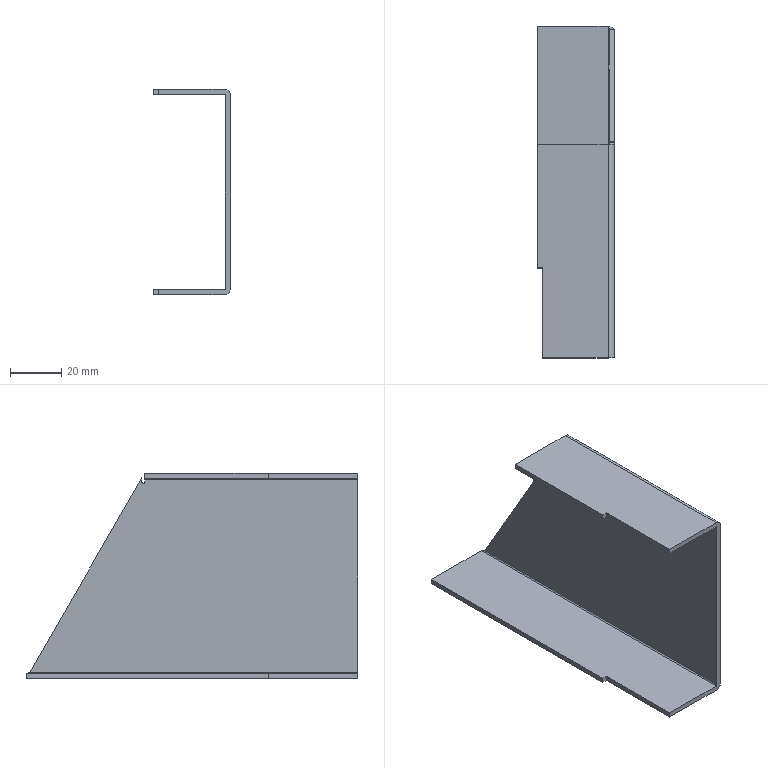Part | STEP file | Guard Rib 3 | 1 solid | 24 faces | box 30 x 129.355 x 80 mm | volume 28343 mm3 | plane 17 | cylinder 6 | spline 1 | commonest cylinder face diameters 1 x4 5 x2
STEP:
#1=CARTESIAN_POINT('',(-2.,-23.29,-481.044));
#2=VERTEX_POINT('',#1);
#3=CARTESIAN_POINT('',(-2.,-22.79,-480.544));
#4=VERTEX_POINT('',#3);
#5=CARTESIAN_POINT('',(-2.,-23.29,-480.544));
#6=DIRECTION('',(1.,0.,0.));
#7=DIRECTION('',(0.,0.,-1.));
#8=AXIS2_PLACEMENT_3D('',#5,#6,#7);
#9=CIRCLE('',#8,0.5);
#10=EDGE_CURVE('',#2,#4,#9,.T.);
#11=ORIENTED_EDGE('',*,*,#10,.F.);
#12=CARTESIAN_POINT('',(0.,-23.29,-481.044));
#13=VERTEX_POINT('',#12);
#14=CARTESIAN_POINT('',(-2.,-23.29,-481.044));
#15=DIRECTION('',(1.,0.,0.));
#16=VECTOR('',#15,1000.);
#17=LINE('',#14,#16);
#18=EDGE_CURVE('',#2,#13,#17,.T.);
#19=ORIENTED_EDGE('',*,*,#18,.T.);
#20=CARTESIAN_POINT('',(0.,-22.79,-480.544));
#21=VERTEX_POINT('',#20);
#22=CARTESIAN_POINT('',(0.,-23.29,-480.544));
#23=DIRECTION('',(1.,0.,0.));
#24=DIRECTION('',(0.,0.,-1.));
#25=AXIS2_PLACEMENT_3D('',#22,#23,#24);
#26=CIRCLE('',#25,0.5);
#27=EDGE_CURVE('',#13,#21,#26,.T.);
#28=ORIENTED_EDGE('',*,*,#27,.T.);
#29=CARTESIAN_POINT('',(-2.,-22.79,-480.544));
#30=DIRECTION('',(1.,0.,0.));
#31=VECTOR('',#30,1000.);
#32=LINE('',#29,#31);
#33=EDGE_CURVE('',#4,#21,#32,.T.);
#34=ORIENTED_EDGE('',*,*,#33,.F.);
#35=EDGE_LOOP('',(#11,#19,#28,#34));
#36=FACE_OUTER_BOUND('',#35,.T.);
#37=CARTESIAN_POINT('',(-2.,-23.29,-480.544));
#38=DIRECTION('',(1.,0.,0.));
#39=DIRECTION('',(0.,0.,-1.));
#40=AXIS2_PLACEMENT_3D('',#37,#38,#39);
#41=CYLINDRICAL_SURFACE('',#40,0.5);
#42=ADVANCED_FACE('',(#36),#41,.F.);
#43=CARTESIAN_POINT('',(-2.,-23.79,-480.544));
#44=VERTEX_POINT('',#43);
#45=CARTESIAN_POINT('',(-2.,-23.79,-479.544));
#46=VERTEX_POINT('',#45);
#47=CARTESIAN_POINT('',(-2.,-23.79,-480.544));
#48=DIRECTION('',(0.,0.,1.));
#49=VECTOR('',#48,1000.);
#50=LINE('',#47,#49);
#51=EDGE_CURVE('',#44,#46,#50,.T.);
#52=ORIENTED_EDGE('',*,*,#51,.F.);
#53=CARTESIAN_POINT('',(-2.,-23.29,-480.544));
#54=DIRECTION('',(1.,0.,0.));
#55=DIRECTION('',(0.,0.,-1.));
#56=AXIS2_PLACEMENT_3D('',#53,#54,#55);
#57=CIRCLE('',#56,0.5);
#58=EDGE_CURVE('',#44,#2,#57,.T.);
#59=ORIENTED_EDGE('',*,*,#58,.T.);
#60=ORIENTED_EDGE('',*,*,#10,.T.);
#61=CARTESIAN_POINT('',(-2.,-22.79,-478.776));
#62=VERTEX_POINT('',#61);
#63=CARTESIAN_POINT('',(-2.,-22.79,0.));
#64=DIRECTION('',(0.,0.,1.));
#65=VECTOR('',#64,1000.);
#66=LINE('',#63,#65);
#67=EDGE_CURVE('',#4,#62,#66,.T.);
#68=ORIENTED_EDGE('',*,*,#67,.T.);
#69=CARTESIAN_POINT('',(-2.,20.955,-554.544));
#70=VERTEX_POINT('',#69);
#71=CARTESIAN_POINT('',(-2.,-22.79,-478.776));
#72=DIRECTION('',(0.,0.5,-0.866));
#73=VECTOR('',#72,1000.);
#74=LINE('',#71,#73);
#75=EDGE_CURVE('',#62,#70,#74,.T.);
#76=ORIENTED_EDGE('',*,*,#75,.T.);
#77=CARTESIAN_POINT('',(-2.,-106.957,-554.544));
#78=VERTEX_POINT('',#77);
#79=CARTESIAN_POINT('',(-2.,0.,-554.544));
#80=DIRECTION('',(0.,-1.,0.));
#81=VECTOR('',#80,1000.);
#82=LINE('',#79,#81);
#83=EDGE_CURVE('',#70,#78,#82,.T.);
#84=ORIENTED_EDGE('',*,*,#83,.T.);
#85=CARTESIAN_POINT('',(-2.,-106.957,-479.544));
#86=VERTEX_POINT('',#85);
#87=CARTESIAN_POINT('',(-2.,-106.957,0.));
#88=DIRECTION('',(0.,0.,1.));
#89=VECTOR('',#88,1000.);
#90=LINE('',#87,#89);
#91=EDGE_CURVE('',#78,#86,#90,.T.);
#92=ORIENTED_EDGE('',*,*,#91,.T.);
#93=CARTESIAN_POINT('',(-2.,0.,-479.544));
#94=DIRECTION('',(0.,1.,0.));
#95=VECTOR('',#94,1000.);
#96=LINE('',#93,#95);
#97=EDGE_CURVE('',#86,#46,#96,.T.);
#98=ORIENTED_EDGE('',*,*,#97,.T.);
#99=EDGE_LOOP('',(#52,#59,#60,#68,#76,#84,#92,#98));
#100=FACE_OUTER_BOUND('',#99,.T.);
#101=CARTESIAN_POINT('',(-2.,0.,0.));
#102=DIRECTION('',(-1.,0.,0.));
#103=DIRECTION('',(0.,0.,1.));
#104=AXIS2_PLACEMENT_3D('',#101,#102,#103);
#105=PLANE('',#104);
#106=ADVANCED_FACE('',(#100),#105,.T.);
#107=CARTESIAN_POINT('',(-2.5,-106.957,-479.044));
#108=VERTEX_POINT('',#107);
#109=CARTESIAN_POINT('',(-2.5,-106.957,-479.544));
#110=DIRECTION('',(0.,1.,0.));
#111=DIRECTION('',(0.,0.,1.));
#112=AXIS2_PLACEMENT_3D('',#109,#110,#111);
#113=CIRCLE('',#112,0.5);
#114=EDGE_CURVE('',#108,#86,#113,.T.);
#115=ORIENTED_EDGE('',*,*,#114,.F.);
#116=CARTESIAN_POINT('',(-2.5,-23.79,-479.044));
#117=VERTEX_POINT('',#116);
#118=CARTESIAN_POINT('',(-2.5,-23.79,-479.044));
#119=DIRECTION('',(0.,-1.,0.));
#120=VECTOR('',#119,1000.);
#121=LINE('',#118,#120);
#122=EDGE_CURVE('',#117,#108,#121,.T.);
#123=ORIENTED_EDGE('',*,*,#122,.F.);
#124=CARTESIAN_POINT('',(-2.5,-23.79,-479.544));
#125=DIRECTION('',(0.,1.,0.));
#126=DIRECTION('',(0.,0.,1.));
#127=AXIS2_PLACEMENT_3D('',#124,#125,#126);
#128=CIRCLE('',#127,0.5);
#129=EDGE_CURVE('',#117,#46,#128,.T.);
#130=ORIENTED_EDGE('',*,*,#129,.T.);
#131=ORIENTED_EDGE('',*,*,#97,.F.);
#132=EDGE_LOOP('',(#115,#123,#130,#131));
#133=FACE_OUTER_BOUND('',#132,.T.);
#134=CARTESIAN_POINT('',(-2.5,-23.79,-479.544));
#135=DIRECTION('',(0.,1.,0.));
#136=DIRECTION('',(0.,0.,1.));
#137=AXIS2_PLACEMENT_3D('',#134,#135,#136);
#138=CYLINDRICAL_SURFACE('',#137,0.5);
#139=ADVANCED_FACE('',(#133),#138,.F.);
#140=ORIENTED_EDGE('',*,*,#91,.F.);
#141=CARTESIAN_POINT('',(-2.5,-106.957,-555.044));
#142=VERTEX_POINT('',#141);
#143=CARTESIAN_POINT('',(-2.5,-106.957,-554.544));
#144=DIRECTION('',(0.,1.,0.));
#145=DIRECTION('',(0.,0.,-1.));
#146=AXIS2_PLACEMENT_3D('',#143,#144,#145);
#147=CIRCLE('',#146,0.5);
#148=EDGE_CURVE('',#78,#142,#147,.T.);
#149=ORIENTED_EDGE('',*,*,#148,.T.);
#150=CARTESIAN_POINT('',(-28.,-106.957,-555.044));
#151=VERTEX_POINT('',#150);
#152=CARTESIAN_POINT('',(0.,-106.957,-555.044));
#153=DIRECTION('',(1.,0.,0.));
#154=VECTOR('',#153,1000.);
#155=LINE('',#152,#154);
#156=EDGE_CURVE('',#151,#142,#155,.T.);
#157=ORIENTED_EDGE('',*,*,#156,.F.);
#158=CARTESIAN_POINT('',(-28.,-106.957,-557.044));
#159=VERTEX_POINT('',#158);
#160=CARTESIAN_POINT('',(-28.,-106.957,-557.044));
#161=DIRECTION('',(0.,0.,1.));
#162=VECTOR('',#161,1000.);
#163=LINE('',#160,#162);
#164=EDGE_CURVE('',#159,#151,#163,.T.);
#165=ORIENTED_EDGE('',*,*,#164,.F.);
#166=CARTESIAN_POINT('',(-2.5,-106.957,-557.044));
#167=VERTEX_POINT('',#166);
#168=CARTESIAN_POINT('',(-30.,-106.957,-557.044));
#169=DIRECTION('',(-1.,0.,0.));
#170=VECTOR('',#169,1000.);
#171=LINE('',#168,#170);
#172=EDGE_CURVE('',#167,#159,#171,.T.);
#173=ORIENTED_EDGE('',*,*,#172,.F.);
#174=CARTESIAN_POINT('',(0.,-106.957,-554.544));
#175=VERTEX_POINT('',#174);
#176=CARTESIAN_POINT('',(-2.5,-106.957,-554.544));
#177=DIRECTION('',(0.,1.,0.));
#178=DIRECTION('',(0.,0.,-1.));
#179=AXIS2_PLACEMENT_3D('',#176,#177,#178);
#180=CIRCLE('',#179,2.5);
#181=EDGE_CURVE('',#175,#167,#180,.T.);
#182=ORIENTED_EDGE('',*,*,#181,.F.);
#183=CARTESIAN_POINT('',(0.,-106.957,-479.544));
#184=VERTEX_POINT('',#183);
#185=CARTESIAN_POINT('',(0.,-106.957,-477.044));
#186=DIRECTION('',(0.,0.,1.));
#187=VECTOR('',#186,1000.);
#188=LINE('',#185,#187);
#189=EDGE_CURVE('',#175,#184,#188,.T.);
#190=ORIENTED_EDGE('',*,*,#189,.T.);
#191=CARTESIAN_POINT('',(-2.5,-106.957,-477.044));
#192=VERTEX_POINT('',#191);
#193=CARTESIAN_POINT('',(-2.5,-106.957,-479.544));
#194=DIRECTION('',(0.,-1.,0.));
#195=DIRECTION('',(0.,0.,1.));
#196=AXIS2_PLACEMENT_3D('',#193,#194,#195);
#197=CIRCLE('',#196,2.5);
#198=EDGE_CURVE('',#184,#192,#197,.T.);
#199=ORIENTED_EDGE('',*,*,#198,.T.);
#200=CARTESIAN_POINT('',(-28.,-106.957,-477.044));
#201=VERTEX_POINT('',#200);
#202=CARTESIAN_POINT('',(-2.,-106.957,-477.044));
#203=DIRECTION('',(1.,0.,0.));
#204=VECTOR('',#203,1000.);
#205=LINE('',#202,#204);
#206=EDGE_CURVE('',#201,#192,#205,.T.);
#207=ORIENTED_EDGE('',*,*,#206,.F.);
#208=CARTESIAN_POINT('',(-28.,-106.957,-479.044));
#209=VERTEX_POINT('',#208);
#210=CARTESIAN_POINT('',(-28.,-106.957,-477.044));
#211=DIRECTION('',(0.,0.,1.));
#212=VECTOR('',#211,1000.);
#213=LINE('',#210,#212);
#214=EDGE_CURVE('',#209,#201,#213,.T.);
#215=ORIENTED_EDGE('',*,*,#214,.F.);
#216=CARTESIAN_POINT('',(0.,-106.957,-479.044));
#217=DIRECTION('',(-1.,0.,0.));
#218=VECTOR('',#217,1000.);
#219=LINE('',#216,#218);
#220=EDGE_CURVE('',#108,#209,#219,.T.);
#221=ORIENTED_EDGE('',*,*,#220,.F.);
#222=ORIENTED_EDGE('',*,*,#114,.T.);
#223=EDGE_LOOP('',(#140,#149,#157,#165,#173,#182,#190,#199,#207,#215,#221,#222));
#224=FACE_OUTER_BOUND('',#223,.T.);
#225=CARTESIAN_POINT('',(-2.,-106.957,-477.044));
#226=DIRECTION('',(0.,-1.,0.));
#227=DIRECTION('',(0.,0.,-1.));
#228=AXIS2_PLACEMENT_3D('',#225,#226,#227);
#229=PLANE('',#228);
#230=ADVANCED_FACE('',(#224),#229,.T.);
#231=CARTESIAN_POINT('',(-2.5,22.398,-555.044));
#232=VERTEX_POINT('',#231);
#233=CARTESIAN_POINT('',(-2.,20.955,-554.544));
#234=CARTESIAN_POINT('',(-2.,21.076,-554.61));
#235=CARTESIAN_POINT('',(-2.013,21.196,-554.675));
#236=CARTESIAN_POINT('',(-2.063,21.435,-554.795));
#237=CARTESIAN_POINT('',(-2.1,21.556,-554.851));
#238=CARTESIAN_POINT('',(-2.239,21.918,-554.99));
#239=CARTESIAN_POINT('',(-2.368,22.155,-555.044));
#240=CARTESIAN_POINT('',(-2.5,22.398,-555.044));
#241=B_SPLINE_CURVE_WITH_KNOTS('',3,(#233,#234,#235,#236,#237,#238,#239,#240),.UNSPECIFIED.,.F.,.F.,(4,2,2,4),(0.,0.0004085,0.0008171,0.001634),.UNSPECIFIED.);
#242=EDGE_CURVE('',#70,#232,#241,.T.);
#243=ORIENTED_EDGE('',*,*,#242,.T.);
#244=CARTESIAN_POINT('',(-2.5,-106.957,-555.044));
#245=DIRECTION('',(0.,1.,0.));
#246=VECTOR('',#245,1000.);
#247=LINE('',#244,#246);
#248=EDGE_CURVE('',#142,#232,#247,.T.);
#249=ORIENTED_EDGE('',*,*,#248,.F.);
#250=ORIENTED_EDGE('',*,*,#148,.F.);
#251=ORIENTED_EDGE('',*,*,#83,.F.);
#252=EDGE_LOOP('',(#243,#249,#250,#251));
#253=FACE_OUTER_BOUND('',#252,.T.);
#254=CARTESIAN_POINT('',(-2.5,-106.957,-554.544));
#255=DIRECTION('',(0.,-1.,0.));
#256=DIRECTION('',(0.,0.,-1.));
#257=AXIS2_PLACEMENT_3D('',#254,#255,#256);
#258=CYLINDRICAL_SURFACE('',#257,0.5);
#259=ADVANCED_FACE('',(#253),#258,.F.);
#260=CARTESIAN_POINT('',(0.,-22.79,-478.776));
#261=VERTEX_POINT('',#260);
#262=CARTESIAN_POINT('',(0.,20.955,-554.544));
#263=VERTEX_POINT('',#262);
#264=CARTESIAN_POINT('',(0.,-23.79,-477.044));
#265=DIRECTION('',(0.,0.5,-0.866));
#266=VECTOR('',#265,1000.);
#267=LINE('',#264,#266);
#268=EDGE_CURVE('',#261,#263,#267,.T.);
#269=ORIENTED_EDGE('',*,*,#268,.T.);
#270=CARTESIAN_POINT('',(-2.,20.955,-554.544));
#271=DIRECTION('',(-1.,0.,0.));
#272=VECTOR('',#271,1000.);
#273=LINE('',#270,#272);
#274=EDGE_CURVE('',#263,#70,#273,.T.);
#275=ORIENTED_EDGE('',*,*,#274,.T.);
#276=ORIENTED_EDGE('',*,*,#75,.F.);
#277=CARTESIAN_POINT('',(-2.,-22.79,-478.776));
#278=DIRECTION('',(1.,0.,0.));
#279=VECTOR('',#278,1000.);
#280=LINE('',#277,#279);
#281=EDGE_CURVE('',#62,#261,#280,.T.);
#282=ORIENTED_EDGE('',*,*,#281,.T.);
#283=EDGE_LOOP('',(#269,#275,#276,#282));
#284=FACE_OUTER_BOUND('',#283,.T.);
#285=CARTESIAN_POINT('',(-2.,-23.79,-477.044));
#286=DIRECTION('',(0.,0.866,0.5));
#287=DIRECTION('',(0.,-0.5,0.866));
#288=AXIS2_PLACEMENT_3D('',#285,#286,#287);
#289=PLANE('',#288);
#290=ADVANCED_FACE('',(#284),#289,.T.);
#291=ORIENTED_EDGE('',*,*,#281,.F.);
#292=ORIENTED_EDGE('',*,*,#67,.F.);
#293=ORIENTED_EDGE('',*,*,#33,.T.);
#294=CARTESIAN_POINT('',(0.,-22.79,-478.776));
#295=DIRECTION('',(0.,0.,1.));
#296=VECTOR('',#295,1000.);
#297=LINE('',#294,#296);
#298=EDGE_CURVE('',#21,#261,#297,.T.);
#299=ORIENTED_EDGE('',*,*,#298,.T.);
#300=EDGE_LOOP('',(#291,#292,#293,#299));
#301=FACE_OUTER_BOUND('',#300,.T.);
#302=CARTESIAN_POINT('',(-2.,-22.79,-478.776));
#303=DIRECTION('',(0.,-1.,0.));
#304=DIRECTION('',(0.,0.,-1.));
#305=AXIS2_PLACEMENT_3D('',#302,#303,#304);
#306=PLANE('',#305);
#307=ADVANCED_FACE('',(#301),#306,.T.);
#308=ORIENTED_EDGE('',*,*,#122,.T.);
#309=ORIENTED_EDGE('',*,*,#220,.T.);
#310=CARTESIAN_POINT('',(-28.,-71.957,-479.044));
#311=VERTEX_POINT('',#310);
#312=CARTESIAN_POINT('',(-28.,0.,-479.044));
#313=DIRECTION('',(0.,1.,0.));
#314=VECTOR('',#313,1000.);
#315=LINE('',#312,#314);
#316=EDGE_CURVE('',#209,#311,#315,.T.);
#317=ORIENTED_EDGE('',*,*,#316,.T.);
#318=CARTESIAN_POINT('',(-30.,-71.957,-479.044));
#319=VERTEX_POINT('',#318);
#320=CARTESIAN_POINT('',(0.,-71.957,-479.044));
#321=DIRECTION('',(-1.,0.,0.));
#322=VECTOR('',#321,1000.);
#323=LINE('',#320,#322);
#324=EDGE_CURVE('',#311,#319,#323,.T.);
#325=ORIENTED_EDGE('',*,*,#324,.T.);
#326=CARTESIAN_POINT('',(-30.,-23.79,-479.044));
#327=VERTEX_POINT('',#326);
#328=CARTESIAN_POINT('',(-30.,0.,-479.044));
#329=DIRECTION('',(0.,1.,0.));
#330=VECTOR('',#329,1000.);
#331=LINE('',#328,#330);
#332=EDGE_CURVE('',#319,#327,#331,.T.);
#333=ORIENTED_EDGE('',*,*,#332,.T.);
#334=CARTESIAN_POINT('',(0.,-23.79,-479.044));
#335=DIRECTION('',(1.,0.,0.));
#336=VECTOR('',#335,1000.);
#337=LINE('',#334,#336);
#338=EDGE_CURVE('',#327,#117,#337,.T.);
#339=ORIENTED_EDGE('',*,*,#338,.T.);
#340=EDGE_LOOP('',(#308,#309,#317,#325,#333,#339));
#341=FACE_OUTER_BOUND('',#340,.T.);
#342=CARTESIAN_POINT('',(0.,0.,-479.044));
#343=DIRECTION('',(0.,0.,-1.));
#344=DIRECTION('',(-1.,0.,0.));
#345=AXIS2_PLACEMENT_3D('',#342,#343,#344);
#346=PLANE('',#345);
#347=ADVANCED_FACE('',(#341),#346,.T.);
#348=CARTESIAN_POINT('',(0.,-23.79,-480.544));
#349=VERTEX_POINT('',#348);
#350=CARTESIAN_POINT('',(0.,-23.29,-480.544));
#351=DIRECTION('',(1.,0.,0.));
#352=DIRECTION('',(0.,0.,-1.));
#353=AXIS2_PLACEMENT_3D('',#350,#351,#352);
#354=CIRCLE('',#353,0.5);
#355=EDGE_CURVE('',#349,#13,#354,.T.);
#356=ORIENTED_EDGE('',*,*,#355,.F.);
#357=CARTESIAN_POINT('',(0.,-23.79,-479.544));
#358=VERTEX_POINT('',#357);
#359=CARTESIAN_POINT('',(0.,-23.79,-480.544));
#360=DIRECTION('',(0.,0.,-1.));
#361=VECTOR('',#360,1000.);
#362=LINE('',#359,#361);
#363=EDGE_CURVE('',#358,#349,#362,.T.);
#364=ORIENTED_EDGE('',*,*,#363,.F.);
#365=CARTESIAN_POINT('',(0.,0.,-479.544));
#366=DIRECTION('',(0.,1.,0.));
#367=VECTOR('',#366,1000.);
#368=LINE('',#365,#367);
#369=EDGE_CURVE('',#184,#358,#368,.T.);
#370=ORIENTED_EDGE('',*,*,#369,.F.);
#371=ORIENTED_EDGE('',*,*,#189,.F.);
#372=CARTESIAN_POINT('',(0.,0.,-554.544));
#373=DIRECTION('',(0.,-1.,0.));
#374=VECTOR('',#373,1000.);
#375=LINE('',#372,#374);
#376=EDGE_CURVE('',#263,#175,#375,.T.);
#377=ORIENTED_EDGE('',*,*,#376,.F.);
#378=ORIENTED_EDGE('',*,*,#268,.F.);
#379=ORIENTED_EDGE('',*,*,#298,.F.);
#380=ORIENTED_EDGE('',*,*,#27,.F.);
#381=EDGE_LOOP('',(#356,#364,#370,#371,#377,#378,#379,#380));
#382=FACE_OUTER_BOUND('',#381,.T.);
#383=CARTESIAN_POINT('',(0.,0.,0.));
#384=DIRECTION('',(-1.,0.,0.));
#385=DIRECTION('',(0.,0.,1.));
#386=AXIS2_PLACEMENT_3D('',#383,#384,#385);
#387=PLANE('',#386);
#388=ADVANCED_FACE('',(#382),#387,.F.);
#389=CARTESIAN_POINT('',(-30.,22.398,-555.044));
#390=VERTEX_POINT('',#389);
#391=CARTESIAN_POINT('',(-30.,-71.957,-555.044));
#392=VERTEX_POINT('',#391);
#393=CARTESIAN_POINT('',(-30.,0.,-555.044));
#394=DIRECTION('',(0.,-1.,0.));
#395=VECTOR('',#394,1000.);
#396=LINE('',#393,#395);
#397=EDGE_CURVE('',#390,#392,#396,.T.);
#398=ORIENTED_EDGE('',*,*,#397,.T.);
#399=CARTESIAN_POINT('',(-28.,-71.957,-555.044));
#400=VERTEX_POINT('',#399);
#401=CARTESIAN_POINT('',(0.,-71.957,-555.044));
#402=DIRECTION('',(1.,0.,0.));
#403=VECTOR('',#402,1000.);
#404=LINE('',#401,#403);
#405=EDGE_CURVE('',#392,#400,#404,.T.);
#406=ORIENTED_EDGE('',*,*,#405,.T.);
#407=CARTESIAN_POINT('',(-28.,0.,-555.044));
#408=DIRECTION('',(0.,-1.,0.));
#409=VECTOR('',#408,1000.);
#410=LINE('',#407,#409);
#411=EDGE_CURVE('',#400,#151,#410,.T.);
#412=ORIENTED_EDGE('',*,*,#411,.T.);
#413=ORIENTED_EDGE('',*,*,#156,.T.);
#414=ORIENTED_EDGE('',*,*,#248,.T.);
#415=CARTESIAN_POINT('',(0.,22.398,-555.044));
#416=DIRECTION('',(-1.,0.,0.));
#417=VECTOR('',#416,1000.);
#418=LINE('',#415,#417);
#419=EDGE_CURVE('',#232,#390,#418,.T.);
#420=ORIENTED_EDGE('',*,*,#419,.T.);
#421=EDGE_LOOP('',(#398,#406,#412,#413,#414,#420));
#422=FACE_OUTER_BOUND('',#421,.T.);
#423=CARTESIAN_POINT('',(0.,0.,-555.044));
#424=DIRECTION('',(0.,0.,1.));
#425=DIRECTION('',(1.,0.,0.));
#426=AXIS2_PLACEMENT_3D('',#423,#424,#425);
#427=PLANE('',#426);
#428=ADVANCED_FACE('',(#422),#427,.T.);
#429=ORIENTED_EDGE('',*,*,#242,.F.);
#430=ORIENTED_EDGE('',*,*,#274,.F.);
#431=CARTESIAN_POINT('',(-2.5,22.398,-557.044));
#432=VERTEX_POINT('',#431);
#433=CARTESIAN_POINT('',(-2.5,22.398,-557.044));
#434=CARTESIAN_POINT('',(-2.17,22.277,-557.044));
#435=CARTESIAN_POINT('',(-1.85,22.159,-556.98));
#436=CARTESIAN_POINT('',(-1.393,21.977,-556.791));
#437=CARTESIAN_POINT('',(-1.248,21.918,-556.714));
#438=CARTESIAN_POINT('',(-0.9774,21.798,-556.533));
#439=CARTESIAN_POINT('',(-0.8497,21.737,-556.429));
#440=CARTESIAN_POINT('',(-0.6169,21.617,-556.196));
#441=CARTESIAN_POINT('',(-0.5135,21.557,-556.07));
#442=CARTESIAN_POINT('',(-0.3321,21.437,-555.799));
#443=CARTESIAN_POINT('',(-0.2536,21.376,-555.653));
#444=CARTESIAN_POINT('',(-0.128,21.256,-555.35));
#445=CARTESIAN_POINT('',(-0.08064,21.196,-555.194));
#446=CARTESIAN_POINT('',(-0.01656,21.076,-554.874));
#447=CARTESIAN_POINT('',(0.,21.015,-554.709));
#448=CARTESIAN_POINT('',(0.,20.955,-554.544));
#449=B_SPLINE_CURVE_WITH_KNOTS('',3,(#433,#434,#435,#436,#437,#438,#439,#440,#441,#442,#443,#444,#445,#446,#447,#448),.UNSPECIFIED.,.F.,.F.,(4,2,2,2,2,2,2,4),(0.,0.001038,0.001557,0.002076,0.002595,0.003114,0.003633,0.004151),.UNSPECIFIED.);
#450=EDGE_CURVE('',#432,#263,#449,.T.);
#451=ORIENTED_EDGE('',*,*,#450,.F.);
#452=CARTESIAN_POINT('',(-2.5,22.398,-556.043));
#453=DIRECTION('',(0.,0.,-1.));
#454=VECTOR('',#453,1000.);
#455=LINE('',#452,#454);
#456=EDGE_CURVE('',#232,#432,#455,.T.);
#457=ORIENTED_EDGE('',*,*,#456,.F.);
#458=EDGE_LOOP('',(#429,#430,#451,#457));
#459=FACE_OUTER_BOUND('',#458,.T.);
#460=CARTESIAN_POINT('',(0.02,20.955,-554.544));
#461=CARTESIAN_POINT('',(0.02,21.075,-554.874));
#462=CARTESIAN_POINT('',(-0.04559,21.195,-555.203));
#463=CARTESIAN_POINT('',(-0.2981,21.436,-555.813));
#464=CARTESIAN_POINT('',(-0.4848,21.556,-556.092));
#465=CARTESIAN_POINT('',(-0.9513,21.797,-556.559));
#466=CARTESIAN_POINT('',(-1.231,21.917,-556.746));
#467=CARTESIAN_POINT('',(-1.84,22.158,-556.998));
#468=CARTESIAN_POINT('',(-2.17,22.278,-557.064));
#469=CARTESIAN_POINT('',(-2.5,22.398,-557.064));
#470=CARTESIAN_POINT('',(0.,20.955,-554.544));
#471=CARTESIAN_POINT('',(0.,21.075,-554.871));
#472=CARTESIAN_POINT('',(-0.06507,21.195,-555.198));
#473=CARTESIAN_POINT('',(-0.3155,21.436,-555.803));
#474=CARTESIAN_POINT('',(-0.5008,21.556,-556.08));
#475=CARTESIAN_POINT('',(-0.9636,21.797,-556.543));
#476=CARTESIAN_POINT('',(-1.241,21.917,-556.728));
#477=CARTESIAN_POINT('',(-1.846,22.158,-556.979));
#478=CARTESIAN_POINT('',(-2.173,22.278,-557.044));
#479=CARTESIAN_POINT('',(-2.5,22.398,-557.044));
#480=CARTESIAN_POINT('',(-2.,20.955,-554.544));
#481=CARTESIAN_POINT('',(-2.,21.075,-554.609));
#482=CARTESIAN_POINT('',(-2.013,21.195,-554.674));
#483=CARTESIAN_POINT('',(-2.063,21.436,-554.795));
#484=CARTESIAN_POINT('',(-2.1,21.556,-554.851));
#485=CARTESIAN_POINT('',(-2.193,21.797,-554.943));
#486=CARTESIAN_POINT('',(-2.248,21.917,-554.98));
#487=CARTESIAN_POINT('',(-2.369,22.158,-555.031));
#488=CARTESIAN_POINT('',(-2.435,22.278,-555.044));
#489=CARTESIAN_POINT('',(-2.5,22.398,-555.044));
#490=CARTESIAN_POINT('',(-2.02,20.955,-554.544));
#491=CARTESIAN_POINT('',(-2.02,21.075,-554.606));
#492=CARTESIAN_POINT('',(-2.033,21.195,-554.669));
#493=CARTESIAN_POINT('',(-2.081,21.436,-554.785));
#494=CARTESIAN_POINT('',(-2.116,21.556,-554.838));
#495=CARTESIAN_POINT('',(-2.205,21.797,-554.927));
#496=CARTESIAN_POINT('',(-2.258,21.917,-554.963));
#497=CARTESIAN_POINT('',(-2.374,22.158,-555.011));
#498=CARTESIAN_POINT('',(-2.437,22.278,-555.023));
#499=CARTESIAN_POINT('',(-2.5,22.398,-555.023));
#500=B_SPLINE_SURFACE_WITH_KNOTS('',1,3,((#460,#461,#462,#463,#464,#465,#466,#467,#468,#469),(#470,#471,#472,#473,#474,#475,#476,#477,#478,#479),(#480,#481,#482,#483,#484,#485,#486,#487,#488,#489),(#490,#491,#492,#493,#494,#495,#496,#497,#498,#499)),.UNSPECIFIED.,.F.,.F.,.F.,(2,1,1,2),(4,2,2,2,4),(-0.01,0.,1.,1.01),(0.,0.25,0.5,0.75,1.),.UNSPECIFIED.);
#501=ADVANCED_FACE('',(#459),#500,.F.);
#502=ORIENTED_EDGE('',*,*,#18,.F.);
#503=ORIENTED_EDGE('',*,*,#58,.F.);
#504=CARTESIAN_POINT('',(-2.,-23.79,-480.544));
#505=DIRECTION('',(-1.,0.,0.));
#506=VECTOR('',#505,1000.);
#507=LINE('',#504,#506);
#508=EDGE_CURVE('',#349,#44,#507,.T.);
#509=ORIENTED_EDGE('',*,*,#508,.F.);
#510=ORIENTED_EDGE('',*,*,#355,.T.);
#511=EDGE_LOOP('',(#502,#503,#509,#510));
#512=FACE_OUTER_BOUND('',#511,.T.);
#513=CARTESIAN_POINT('',(-2.,-23.29,-480.544));
#514=DIRECTION('',(1.,0.,0.));
#515=DIRECTION('',(0.,0.,-1.));
#516=AXIS2_PLACEMENT_3D('',#513,#514,#515);
#517=CYLINDRICAL_SURFACE('',#516,0.5);
#518=ADVANCED_FACE('',(#512),#517,.F.);
#519=ORIENTED_EDGE('',*,*,#338,.F.);
#520=CARTESIAN_POINT('',(-30.,-23.79,-477.044));
#521=VERTEX_POINT('',#520);
#522=CARTESIAN_POINT('',(-30.,-23.79,-477.044));
#523=DIRECTION('',(0.,0.,-1.));
#524=VECTOR('',#523,1000.);
#525=LINE('',#522,#524);
#526=EDGE_CURVE('',#521,#327,#525,.T.);
#527=ORIENTED_EDGE('',*,*,#526,.F.);
#528=CARTESIAN_POINT('',(-2.5,-23.79,-477.044));
#529=VERTEX_POINT('',#528);
#530=CARTESIAN_POINT('',(-30.,-23.79,-477.044));
#531=DIRECTION('',(-1.,0.,0.));
#532=VECTOR('',#531,1000.);
#533=LINE('',#530,#532);
#534=EDGE_CURVE('',#529,#521,#533,.T.);
#535=ORIENTED_EDGE('',*,*,#534,.F.);
#536=CARTESIAN_POINT('',(-2.5,-23.79,-479.544));
#537=DIRECTION('',(0.,-1.,0.));
#538=DIRECTION('',(0.,0.,1.));
#539=AXIS2_PLACEMENT_3D('',#536,#537,#538);
#540=CIRCLE('',#539,2.5);
#541=EDGE_CURVE('',#358,#529,#540,.T.);
#542=ORIENTED_EDGE('',*,*,#541,.F.);
#543=ORIENTED_EDGE('',*,*,#363,.T.);
#544=ORIENTED_EDGE('',*,*,#508,.T.);
#545=ORIENTED_EDGE('',*,*,#51,.T.);
#546=ORIENTED_EDGE('',*,*,#129,.F.);
#547=EDGE_LOOP('',(#519,#527,#535,#542,#543,#544,#545,#546));
#548=FACE_OUTER_BOUND('',#547,.T.);
#549=CARTESIAN_POINT('',(-30.,-23.79,-477.044));
#550=DIRECTION('',(0.,-1.,0.));
#551=DIRECTION('',(0.,0.,-1.));
#552=AXIS2_PLACEMENT_3D('',#549,#550,#551);
#553=PLANE('',#552);
#554=ADVANCED_FACE('',(#548),#553,.F.);
#555=CARTESIAN_POINT('',(-30.,-71.957,-477.044));
#556=VERTEX_POINT('',#555);
#557=CARTESIAN_POINT('',(-30.,-71.957,-477.044));
#558=DIRECTION('',(0.,0.,-1.));
#559=VECTOR('',#558,1000.);
#560=LINE('',#557,#559);
#561=EDGE_CURVE('',#556,#319,#560,.T.);
#562=ORIENTED_EDGE('',*,*,#561,.F.);
#563=CARTESIAN_POINT('',(-30.,-106.957,-477.044));
#564=DIRECTION('',(0.,-1.,0.));
#565=VECTOR('',#564,1000.);
#566=LINE('',#563,#565);
#567=EDGE_CURVE('',#521,#556,#566,.T.);
#568=ORIENTED_EDGE('',*,*,#567,.F.);
#569=ORIENTED_EDGE('',*,*,#526,.T.);
#570=ORIENTED_EDGE('',*,*,#332,.F.);
#571=EDGE_LOOP('',(#562,#568,#569,#570));
#572=FACE_OUTER_BOUND('',#571,.T.);
#573=CARTESIAN_POINT('',(-30.,-106.957,-477.044));
#574=DIRECTION('',(1.,0.,0.));
#575=DIRECTION('',(0.,0.,-1.));
#576=AXIS2_PLACEMENT_3D('',#573,#574,#575);
#577=PLANE('',#576);
#578=ADVANCED_FACE('',(#572),#577,.F.);
#579=CARTESIAN_POINT('',(-28.,-71.957,-477.044));
#580=VERTEX_POINT('',#579);
#581=CARTESIAN_POINT('',(-28.,-71.957,-477.044));
#582=DIRECTION('',(0.,0.,-1.));
#583=VECTOR('',#582,1000.);
#584=LINE('',#581,#583);
#585=EDGE_CURVE('',#580,#311,#584,.T.);
#586=ORIENTED_EDGE('',*,*,#585,.F.);
#587=CARTESIAN_POINT('',(-30.,-71.957,-477.044));
#588=DIRECTION('',(1.,0.,0.));
#589=VECTOR('',#588,1000.);
#590=LINE('',#587,#589);
#591=EDGE_CURVE('',#556,#580,#590,.T.);
#592=ORIENTED_EDGE('',*,*,#591,.F.);
#593=ORIENTED_EDGE('',*,*,#561,.T.);
#594=ORIENTED_EDGE('',*,*,#324,.F.);
#595=EDGE_LOOP('',(#586,#592,#593,#594));
#596=FACE_OUTER_BOUND('',#595,.T.);
#597=CARTESIAN_POINT('',(-30.,-71.957,-477.044));
#598=DIRECTION('',(0.,1.,0.));
#599=DIRECTION('',(0.,0.,1.));
#600=AXIS2_PLACEMENT_3D('',#597,#598,#599);
#601=PLANE('',#600);
#602=ADVANCED_FACE('',(#596),#601,.F.);
#603=ORIENTED_EDGE('',*,*,#214,.T.);
#604=CARTESIAN_POINT('',(-28.,-106.957,-477.044));
#605=DIRECTION('',(0.,-1.,0.));
#606=VECTOR('',#605,1000.);
#607=LINE('',#604,#606);
#608=EDGE_CURVE('',#580,#201,#607,.T.);
#609=ORIENTED_EDGE('',*,*,#608,.F.);
#610=ORIENTED_EDGE('',*,*,#585,.T.);
#611=ORIENTED_EDGE('',*,*,#316,.F.);
#612=EDGE_LOOP('',(#603,#609,#610,#611));
#613=FACE_OUTER_BOUND('',#612,.T.);
#614=CARTESIAN_POINT('',(-28.,-106.957,-477.044));
#615=DIRECTION('',(1.,0.,0.));
#616=DIRECTION('',(0.,0.,-1.));
#617=AXIS2_PLACEMENT_3D('',#614,#615,#616);
#618=PLANE('',#617);
#619=ADVANCED_FACE('',(#613),#618,.F.);
#620=CARTESIAN_POINT('',(-2.5,-23.79,-477.044));
#621=DIRECTION('',(0.,-1.,0.));
#622=VECTOR('',#621,1000.);
#623=LINE('',#620,#622);
#624=EDGE_CURVE('',#529,#192,#623,.T.);
#625=ORIENTED_EDGE('',*,*,#624,.T.);
#626=ORIENTED_EDGE('',*,*,#198,.F.);
#627=ORIENTED_EDGE('',*,*,#369,.T.);
#628=ORIENTED_EDGE('',*,*,#541,.T.);
#629=EDGE_LOOP('',(#625,#626,#627,#628));
#630=FACE_OUTER_BOUND('',#629,.T.);
#631=CARTESIAN_POINT('',(-2.5,-23.79,-479.544));
#632=DIRECTION('',(0.,1.,0.));
#633=DIRECTION('',(0.,0.,1.));
#634=AXIS2_PLACEMENT_3D('',#631,#632,#633);
#635=CYLINDRICAL_SURFACE('',#634,2.5);
#636=ADVANCED_FACE('',(#630),#635,.T.);
#637=CARTESIAN_POINT('',(-2.5,-106.957,-557.044));
#638=DIRECTION('',(0.,1.,0.));
#639=VECTOR('',#638,1000.);
#640=LINE('',#637,#639);
#641=EDGE_CURVE('',#167,#432,#640,.T.);
#642=ORIENTED_EDGE('',*,*,#641,.T.);
#643=ORIENTED_EDGE('',*,*,#450,.T.);
#644=ORIENTED_EDGE('',*,*,#376,.T.);
#645=ORIENTED_EDGE('',*,*,#181,.T.);
#646=EDGE_LOOP('',(#642,#643,#644,#645));
#647=FACE_OUTER_BOUND('',#646,.T.);
#648=CARTESIAN_POINT('',(-2.5,-106.957,-554.544));
#649=DIRECTION('',(0.,-1.,0.));
#650=DIRECTION('',(0.,0.,-1.));
#651=AXIS2_PLACEMENT_3D('',#648,#649,#650);
#652=CYLINDRICAL_SURFACE('',#651,2.5);
#653=ADVANCED_FACE('',(#647),#652,.T.);
#654=CARTESIAN_POINT('',(-30.,-71.957,-557.044));
#655=VERTEX_POINT('',#654);
#656=CARTESIAN_POINT('',(-30.,-71.957,-477.044));
#657=DIRECTION('',(0.,0.,1.));
#658=VECTOR('',#657,1000.);
#659=LINE('',#656,#658);
#660=EDGE_CURVE('',#655,#392,#659,.T.);
#661=ORIENTED_EDGE('',*,*,#660,.F.);
#662=CARTESIAN_POINT('',(-28.,-71.957,-557.044));
#663=VERTEX_POINT('',#662);
#664=CARTESIAN_POINT('',(-30.,-71.957,-557.044));
#665=DIRECTION('',(-1.,0.,0.));
#666=VECTOR('',#665,1000.);
#667=LINE('',#664,#666);
#668=EDGE_CURVE('',#663,#655,#667,.T.);
#669=ORIENTED_EDGE('',*,*,#668,.F.);
#670=CARTESIAN_POINT('',(-28.,-71.957,-477.044));
#671=DIRECTION('',(0.,0.,-1.));
#672=VECTOR('',#671,1000.);
#673=LINE('',#670,#672);
#674=EDGE_CURVE('',#400,#663,#673,.T.);
#675=ORIENTED_EDGE('',*,*,#674,.F.);
#676=ORIENTED_EDGE('',*,*,#405,.F.);
#677=EDGE_LOOP('',(#661,#669,#675,#676));
#678=FACE_OUTER_BOUND('',#677,.T.);
#679=CARTESIAN_POINT('',(-30.,-71.957,-477.044));
#680=DIRECTION('',(0.,1.,0.));
#681=DIRECTION('',(0.,0.,1.));
#682=AXIS2_PLACEMENT_3D('',#679,#680,#681);
#683=PLANE('',#682);
#684=ADVANCED_FACE('',(#678),#683,.F.);
#685=ORIENTED_EDGE('',*,*,#660,.T.);
#686=ORIENTED_EDGE('',*,*,#397,.F.);
#687=CARTESIAN_POINT('',(-30.,22.398,-557.044));
#688=VERTEX_POINT('',#687);
#689=CARTESIAN_POINT('',(-30.,22.398,-557.044));
#690=DIRECTION('',(0.,0.,1.));
#691=VECTOR('',#690,1000.);
#692=LINE('',#689,#691);
#693=EDGE_CURVE('',#688,#390,#692,.T.);
#694=ORIENTED_EDGE('',*,*,#693,.F.);
#695=CARTESIAN_POINT('',(-30.,22.398,-557.044));
#696=DIRECTION('',(0.,1.,0.));
#697=VECTOR('',#696,1000.);
#698=LINE('',#695,#697);
#699=EDGE_CURVE('',#655,#688,#698,.T.);
#700=ORIENTED_EDGE('',*,*,#699,.F.);
#701=EDGE_LOOP('',(#685,#686,#694,#700));
#702=FACE_OUTER_BOUND('',#701,.T.);
#703=CARTESIAN_POINT('',(-30.,22.398,-557.044));
#704=DIRECTION('',(1.,0.,0.));
#705=DIRECTION('',(0.,0.,-1.));
#706=AXIS2_PLACEMENT_3D('',#703,#704,#705);
#707=PLANE('',#706);
#708=ADVANCED_FACE('',(#702),#707,.F.);
#709=CARTESIAN_POINT('',(-2.,22.398,-557.044));
#710=DIRECTION('',(1.,0.,0.));
#711=VECTOR('',#710,1000.);
#712=LINE('',#709,#711);
#713=EDGE_CURVE('',#688,#432,#712,.T.);
#714=ORIENTED_EDGE('',*,*,#713,.F.);
#715=ORIENTED_EDGE('',*,*,#693,.T.);
#716=ORIENTED_EDGE('',*,*,#419,.F.);
#717=ORIENTED_EDGE('',*,*,#456,.T.);
#718=EDGE_LOOP('',(#714,#715,#716,#717));
#719=FACE_OUTER_BOUND('',#718,.T.);
#720=CARTESIAN_POINT('',(-2.,22.398,-557.044));
#721=DIRECTION('',(0.,-1.,0.));
#722=DIRECTION('',(0.,0.,-1.));
#723=AXIS2_PLACEMENT_3D('',#720,#721,#722);
#724=PLANE('',#723);
#725=ADVANCED_FACE('',(#719),#724,.F.);
#726=ORIENTED_EDGE('',*,*,#674,.T.);
#727=CARTESIAN_POINT('',(-28.,-106.957,-557.044));
#728=DIRECTION('',(0.,1.,0.));
#729=VECTOR('',#728,1000.);
#730=LINE('',#727,#729);
#731=EDGE_CURVE('',#159,#663,#730,.T.);
#732=ORIENTED_EDGE('',*,*,#731,.F.);
#733=ORIENTED_EDGE('',*,*,#164,.T.);
#734=ORIENTED_EDGE('',*,*,#411,.F.);
#735=EDGE_LOOP('',(#726,#732,#733,#734));
#736=FACE_OUTER_BOUND('',#735,.T.);
#737=CARTESIAN_POINT('',(-28.,-106.957,-477.044));
#738=DIRECTION('',(1.,0.,0.));
#739=DIRECTION('',(0.,0.,-1.));
#740=AXIS2_PLACEMENT_3D('',#737,#738,#739);
#741=PLANE('',#740);
#742=ADVANCED_FACE('',(#736),#741,.F.);
#743=ORIENTED_EDGE('',*,*,#608,.T.);
#744=ORIENTED_EDGE('',*,*,#206,.T.);
#745=ORIENTED_EDGE('',*,*,#624,.F.);
#746=ORIENTED_EDGE('',*,*,#534,.T.);
#747=ORIENTED_EDGE('',*,*,#567,.T.);
#748=ORIENTED_EDGE('',*,*,#591,.T.);
#749=EDGE_LOOP('',(#743,#744,#745,#746,#747,#748));
#750=FACE_OUTER_BOUND('',#749,.T.);
#751=CARTESIAN_POINT('',(0.,0.,-477.044));
#752=DIRECTION('',(0.,0.,-1.));
#753=DIRECTION('',(-1.,0.,0.));
#754=AXIS2_PLACEMENT_3D('',#751,#752,#753);
#755=PLANE('',#754);
#756=ADVANCED_FACE('',(#750),#755,.F.);
#757=ORIENTED_EDGE('',*,*,#731,.T.);
#758=ORIENTED_EDGE('',*,*,#668,.T.);
#759=ORIENTED_EDGE('',*,*,#699,.T.);
#760=ORIENTED_EDGE('',*,*,#713,.T.);
#761=ORIENTED_EDGE('',*,*,#641,.F.);
#762=ORIENTED_EDGE('',*,*,#172,.T.);
#763=EDGE_LOOP('',(#757,#758,#759,#760,#761,#762));
#764=FACE_OUTER_BOUND('',#763,.T.);
#765=CARTESIAN_POINT('',(0.,0.,-557.044));
#766=DIRECTION('',(0.,0.,1.));
#767=DIRECTION('',(1.,0.,0.));
#768=AXIS2_PLACEMENT_3D('',#765,#766,#767);
#769=PLANE('',#768);
#770=ADVANCED_FACE('',(#764),#769,.F.);
#771=CLOSED_SHELL('',(#42,#106,#139,#230,#259,#290,#307,#347,#388,#428,#501,#518,#554,#578,#602,#619,#636,#653,#684,#708,#725,#742,#756,#770));
#772=MANIFOLD_SOLID_BREP('',#771);
#773=CARTESIAN_POINT('',(0.,0.,0.));
#774=DIRECTION('',(0.,0.,1.));
#775=DIRECTION('',(1.,0.,0.));
#776=AXIS2_PLACEMENT_3D('',#773,#774,#775);
#777=(LENGTH_UNIT()NAMED_UNIT(*)SI_UNIT(.MILLI.,.METRE.));
#778=UNCERTAINTY_MEASURE_WITH_UNIT(LENGTH_MEASURE(0.00001),#777,'','');
#779=(NAMED_UNIT(*)PLANE_ANGLE_UNIT()SI_UNIT($,.RADIAN.));
#780=(NAMED_UNIT(*)SI_UNIT($,.STERADIAN.)SOLID_ANGLE_UNIT());
#781=(GEOMETRIC_REPRESENTATION_CONTEXT(3)GLOBAL_UNCERTAINTY_ASSIGNED_CONTEXT((#778))GLOBAL_UNIT_ASSIGNED_CONTEXT((#777,#779,#780))REPRESENTATION_CONTEXT('',''));
#782=ADVANCED_BREP_SHAPE_REPRESENTATION('',(#772,#776),#781);